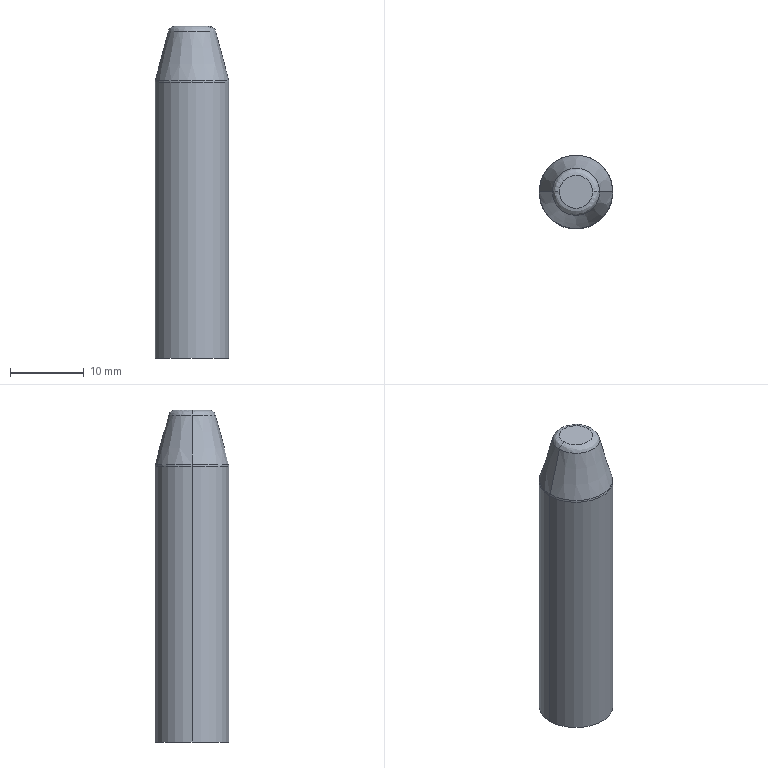Part | STEP file | Guard post | 1 solid | 13 faces | box 10 x 10 x 45 mm | volume 3034 mm3 | spline 4 | cylinder 4 | plane 3 | cone 2 | commonest cylinder face diameters 5 x2 10 x2
STEP:
#1=CARTESIAN_POINT('',(0.,0.,0.));
#2=DIRECTION('',(0.,0.,1.));
#3=DIRECTION('',(1.,0.,0.));
#4=AXIS2_PLACEMENT_3D('',#1,#2,#3);
#5=CARTESIAN_POINT('',(4.966,0.,37.663));
#6=VERTEX_POINT('',#5);
#7=CARTESIAN_POINT('',(-4.966,0.,37.663));
#8=VERTEX_POINT('',#7);
#9=CARTESIAN_POINT('',(0.,0.,37.663));
#10=DIRECTION('',(0.,0.,-1.));
#11=DIRECTION('',(1.,0.,0.));
#12=AXIS2_PLACEMENT_3D('',#9,#10,#11);
#13=CIRCLE('',#12,4.966);
#14=CARTESIAN_POINT('',(-4.966,0.,37.663));
#15=CARTESIAN_POINT('',(-4.966,-9.932,37.663));
#16=CARTESIAN_POINT('',(4.966,-9.932,37.663));
#17=CARTESIAN_POINT('',(4.966,0.,37.663));
#18=CARTESIAN_POINT('',(-4.989,0.,37.579));
#19=CARTESIAN_POINT('',(-4.989,-9.977,37.579));
#20=CARTESIAN_POINT('',(4.989,-9.977,37.579));
#21=CARTESIAN_POINT('',(4.989,0.,37.579));
#22=CARTESIAN_POINT('',(-5.,0.,37.492));
#23=CARTESIAN_POINT('',(-5.,-10.,37.492));
#24=CARTESIAN_POINT('',(5.,-10.,37.492));
#25=CARTESIAN_POINT('',(5.,0.,37.492));
#26=CARTESIAN_POINT('',(-5.,0.,37.404));
#27=CARTESIAN_POINT('',(-5.,-10.,37.404));
#28=CARTESIAN_POINT('',(5.,-10.,37.404));
#29=CARTESIAN_POINT('',(5.,0.,37.404));
#30=(BOUNDED_SURFACE()B_SPLINE_SURFACE(3,3,((#14,#15,#16,#17),(#18,#19,#20,#21),(#22,#23,#24,#25),(#26,#27,#28,#29)),.UNSPECIFIED.,.F.,.F.,.F.)B_SPLINE_SURFACE_WITH_KNOTS((4,4),(4,4),(0.,1.),(0.,1.),.PIECEWISE_BEZIER_KNOTS.)GEOMETRIC_REPRESENTATION_ITEM()RATIONAL_B_SPLINE_SURFACE(((1.,0.3333,0.3333,1.),(0.9943,0.3314,0.3314,0.9943),(0.9943,0.3314,0.3314,0.9943),(1.,0.3333,0.3333,1.)))REPRESENTATION_ITEM('')SURFACE());
#31=CARTESIAN_POINT('',(0.,1.));
#32=CARTESIAN_POINT('',(0.,0.9763));
#33=CARTESIAN_POINT('',(0.,0.9319));
#34=CARTESIAN_POINT('',(0.,0.8733));
#35=CARTESIAN_POINT('',(0.,0.8206));
#36=CARTESIAN_POINT('',(0.,0.7724));
#37=CARTESIAN_POINT('',(0.,0.7279));
#38=CARTESIAN_POINT('',(0.,0.6861));
#39=CARTESIAN_POINT('',(0.,0.6465));
#40=CARTESIAN_POINT('',(0.,0.6086));
#41=CARTESIAN_POINT('',(0.,0.5718));
#42=CARTESIAN_POINT('',(0.,0.5357));
#43=CARTESIAN_POINT('',(0.,0.5));
#44=CARTESIAN_POINT('',(0.,0.4643));
#45=CARTESIAN_POINT('',(0.,0.4282));
#46=CARTESIAN_POINT('',(0.,0.3914));
#47=CARTESIAN_POINT('',(0.,0.3535));
#48=CARTESIAN_POINT('',(0.,0.3139));
#49=CARTESIAN_POINT('',(0.,0.2721));
#50=CARTESIAN_POINT('',(0.,0.2276));
#51=CARTESIAN_POINT('',(0.,0.1794));
#52=CARTESIAN_POINT('',(0.,0.1267));
#53=CARTESIAN_POINT('',(0.,0.06805));
#54=CARTESIAN_POINT('',(0.,0.02375));
#55=CARTESIAN_POINT('',(0.,0.));
#56=B_SPLINE_CURVE_WITH_KNOTS('',3,(#31,#32,#33,#34,#35,#36,#37,#38,#39,#40,#41,#42,#43,#44,#45,#46,#47,#48,#49,#50,#51,#52,#53,#54,#55),.UNSPECIFIED.,.F.,.F.,(4,1,1,1,1,1,1,1,1,1,1,1,1,1,1,1,1,1,1,1,1,1,4),(0.,0.1428,0.2856,0.4284,0.5712,0.714,0.8568,0.9996,1.142,1.285,1.428,1.571,1.714,1.856,1.999,2.142,2.285,2.428,2.57,2.713,2.856,2.999,3.142),.QUASI_UNIFORM_KNOTS.);
#57=(GEOMETRIC_REPRESENTATION_CONTEXT(2)PARAMETRIC_REPRESENTATION_CONTEXT()REPRESENTATION_CONTEXT('',''));
#58=DEFINITIONAL_REPRESENTATION('',(#56),#57);
#59=PCURVE('',#30,#58);
#60=CARTESIAN_POINT('',(0.,0.,37.663));
#61=DIRECTION('',(0.,0.,-1.));
#62=DIRECTION('',(-1.,0.,0.));
#63=AXIS2_PLACEMENT_3D('',#60,#61,#62);
#64=CONICAL_SURFACE('',#63,4.966,0.2618);
#65=CARTESIAN_POINT('',(3.142,0.));
#66=DIRECTION('',(1.,0.));
#67=VECTOR('',#66,1.);
#68=LINE('',#65,#67);
#69=(GEOMETRIC_REPRESENTATION_CONTEXT(2)PARAMETRIC_REPRESENTATION_CONTEXT()REPRESENTATION_CONTEXT('',''));
#70=DEFINITIONAL_REPRESENTATION('',(#68),#69);
#71=PCURVE('',#64,#70);
#72=SURFACE_CURVE('',#13,(#59,#71),.PCURVE_S1.);
#73=EDGE_CURVE('',#6,#8,#72,.T.);
#74=ORIENTED_EDGE('',*,*,#73,.T.);
#75=CARTESIAN_POINT('',(-5.,0.,37.404));
#76=VERTEX_POINT('',#75);
#77=CARTESIAN_POINT('',(-4.,0.,37.404));
#78=DIRECTION('',(0.,-1.,0.));
#79=DIRECTION('',(-1.,0.,0.));
#80=AXIS2_PLACEMENT_3D('',#77,#78,#79);
#81=CIRCLE('',#80,1.);
#82=CARTESIAN_POINT('',(0.,0.));
#83=CARTESIAN_POINT('',(0.01519,0.));
#84=CARTESIAN_POINT('',(0.04557,0.));
#85=CARTESIAN_POINT('',(0.09111,0.));
#86=CARTESIAN_POINT('',(0.1366,0.));
#87=CARTESIAN_POINT('',(0.1821,0.));
#88=CARTESIAN_POINT('',(0.2275,0.));
#89=CARTESIAN_POINT('',(0.273,0.));
#90=CARTESIAN_POINT('',(0.3184,0.));
#91=CARTESIAN_POINT('',(0.3638,0.));
#92=CARTESIAN_POINT('',(0.4092,0.));
#93=CARTESIAN_POINT('',(0.4546,0.));
#94=CARTESIAN_POINT('',(0.5,0.));
#95=CARTESIAN_POINT('',(0.5454,0.));
#96=CARTESIAN_POINT('',(0.5908,0.));
#97=CARTESIAN_POINT('',(0.6362,0.));
#98=CARTESIAN_POINT('',(0.6816,0.));
#99=CARTESIAN_POINT('',(0.727,0.));
#100=CARTESIAN_POINT('',(0.7725,0.));
#101=CARTESIAN_POINT('',(0.8179,0.));
#102=CARTESIAN_POINT('',(0.8634,0.));
#103=CARTESIAN_POINT('',(0.9089,0.));
#104=CARTESIAN_POINT('',(0.9544,0.));
#105=CARTESIAN_POINT('',(0.9848,0.));
#106=CARTESIAN_POINT('',(1.,0.));
#107=B_SPLINE_CURVE_WITH_KNOTS('',3,(#82,#83,#84,#85,#86,#87,#88,#89,#90,#91,#92,#93,#94,#95,#96,#97,#98,#99,#100,#101,#102,#103,#104,#105,#106),.UNSPECIFIED.,.F.,.F.,(4,1,1,1,1,1,1,1,1,1,1,1,1,1,1,1,1,1,1,1,1,1,4),(6.021,6.033,6.045,6.057,6.069,6.081,6.093,6.105,6.117,6.128,6.14,6.152,6.164,6.176,6.188,6.2,6.212,6.224,6.236,6.247,6.259,6.271,6.283),.QUASI_UNIFORM_KNOTS.);
#108=(GEOMETRIC_REPRESENTATION_CONTEXT(2)PARAMETRIC_REPRESENTATION_CONTEXT()REPRESENTATION_CONTEXT('',''));
#109=DEFINITIONAL_REPRESENTATION('',(#107),#108);
#110=PCURVE('',#30,#109);
#111=CARTESIAN_POINT('',(4.966,0.,37.663));
#112=CARTESIAN_POINT('',(4.966,9.932,37.663));
#113=CARTESIAN_POINT('',(-4.966,9.932,37.663));
#114=CARTESIAN_POINT('',(-4.966,0.,37.663));
#115=CARTESIAN_POINT('',(4.989,0.,37.579));
#116=CARTESIAN_POINT('',(4.989,9.977,37.579));
#117=CARTESIAN_POINT('',(-4.989,9.977,37.579));
#118=CARTESIAN_POINT('',(-4.989,0.,37.579));
#119=CARTESIAN_POINT('',(5.,0.,37.492));
#120=CARTESIAN_POINT('',(5.,10.,37.492));
#121=CARTESIAN_POINT('',(-5.,10.,37.492));
#122=CARTESIAN_POINT('',(-5.,0.,37.492));
#123=CARTESIAN_POINT('',(5.,0.,37.404));
#124=CARTESIAN_POINT('',(5.,10.,37.404));
#125=CARTESIAN_POINT('',(-5.,10.,37.404));
#126=CARTESIAN_POINT('',(-5.,0.,37.404));
#127=(BOUNDED_SURFACE()B_SPLINE_SURFACE(3,3,((#111,#112,#113,#114),(#115,#116,#117,#118),(#119,#120,#121,#122),(#123,#124,#125,#126)),.UNSPECIFIED.,.F.,.F.,.F.)B_SPLINE_SURFACE_WITH_KNOTS((4,4),(4,4),(0.,1.),(0.,1.),.PIECEWISE_BEZIER_KNOTS.)GEOMETRIC_REPRESENTATION_ITEM()RATIONAL_B_SPLINE_SURFACE(((1.,0.3333,0.3333,1.),(0.9943,0.3314,0.3314,0.9943),(0.9943,0.3314,0.3314,0.9943),(1.,0.3333,0.3333,1.)))REPRESENTATION_ITEM('')SURFACE());
#128=CARTESIAN_POINT('',(0.,1.));
#129=CARTESIAN_POINT('',(0.01519,1.));
#130=CARTESIAN_POINT('',(0.04557,1.));
#131=CARTESIAN_POINT('',(0.09111,1.));
#132=CARTESIAN_POINT('',(0.1366,1.));
#133=CARTESIAN_POINT('',(0.1821,1.));
#134=CARTESIAN_POINT('',(0.2275,1.));
#135=CARTESIAN_POINT('',(0.273,1.));
#136=CARTESIAN_POINT('',(0.3184,1.));
#137=CARTESIAN_POINT('',(0.3638,1.));
#138=CARTESIAN_POINT('',(0.4092,1.));
#139=CARTESIAN_POINT('',(0.4546,1.));
#140=CARTESIAN_POINT('',(0.5,1.));
#141=CARTESIAN_POINT('',(0.5454,1.));
#142=CARTESIAN_POINT('',(0.5908,1.));
#143=CARTESIAN_POINT('',(0.6362,1.));
#144=CARTESIAN_POINT('',(0.6816,1.));
#145=CARTESIAN_POINT('',(0.727,1.));
#146=CARTESIAN_POINT('',(0.7725,1.));
#147=CARTESIAN_POINT('',(0.8179,1.));
#148=CARTESIAN_POINT('',(0.8634,1.));
#149=CARTESIAN_POINT('',(0.9089,1.));
#150=CARTESIAN_POINT('',(0.9544,1.));
#151=CARTESIAN_POINT('',(0.9848,1.));
#152=CARTESIAN_POINT('',(1.,1.));
#153=B_SPLINE_CURVE_WITH_KNOTS('',3,(#128,#129,#130,#131,#132,#133,#134,#135,#136,#137,#138,#139,#140,#141,#142,#143,#144,#145,#146,#147,#148,#149,#150,#151,#152),.UNSPECIFIED.,.F.,.F.,(4,1,1,1,1,1,1,1,1,1,1,1,1,1,1,1,1,1,1,1,1,1,4),(6.021,6.033,6.045,6.057,6.069,6.081,6.093,6.105,6.117,6.128,6.14,6.152,6.164,6.176,6.188,6.2,6.212,6.224,6.236,6.247,6.259,6.271,6.283),.QUASI_UNIFORM_KNOTS.);
#154=(GEOMETRIC_REPRESENTATION_CONTEXT(2)PARAMETRIC_REPRESENTATION_CONTEXT()REPRESENTATION_CONTEXT('',''));
#155=DEFINITIONAL_REPRESENTATION('',(#153),#154);
#156=PCURVE('',#127,#155);
#157=SURFACE_CURVE('',#81,(#110,#156),.PCURVE_S1.);
#158=EDGE_CURVE('',#8,#76,#157,.T.);
#159=ORIENTED_EDGE('',*,*,#158,.T.);
#160=CARTESIAN_POINT('',(5.,0.,37.404));
#161=VERTEX_POINT('',#160);
#162=CARTESIAN_POINT('',(0.,0.,37.404));
#163=DIRECTION('',(0.,0.,-1.));
#164=DIRECTION('',(-1.,0.,0.));
#165=AXIS2_PLACEMENT_3D('',#162,#163,#164);
#166=CIRCLE('',#165,5.);
#167=CARTESIAN_POINT('',(1.,1.));
#168=CARTESIAN_POINT('',(1.,0.9763));
#169=CARTESIAN_POINT('',(1.,0.9319));
#170=CARTESIAN_POINT('',(1.,0.8733));
#171=CARTESIAN_POINT('',(1.,0.8206));
#172=CARTESIAN_POINT('',(1.,0.7724));
#173=CARTESIAN_POINT('',(1.,0.7279));
#174=CARTESIAN_POINT('',(1.,0.6861));
#175=CARTESIAN_POINT('',(1.,0.6465));
#176=CARTESIAN_POINT('',(1.,0.6086));
#177=CARTESIAN_POINT('',(1.,0.5718));
#178=CARTESIAN_POINT('',(1.,0.5357));
#179=CARTESIAN_POINT('',(1.,0.5));
#180=CARTESIAN_POINT('',(1.,0.4643));
#181=CARTESIAN_POINT('',(1.,0.4282));
#182=CARTESIAN_POINT('',(1.,0.3914));
#183=CARTESIAN_POINT('',(1.,0.3535));
#184=CARTESIAN_POINT('',(1.,0.3139));
#185=CARTESIAN_POINT('',(1.,0.2721));
#186=CARTESIAN_POINT('',(1.,0.2276));
#187=CARTESIAN_POINT('',(1.,0.1794));
#188=CARTESIAN_POINT('',(1.,0.1267));
#189=CARTESIAN_POINT('',(1.,0.06805));
#190=CARTESIAN_POINT('',(1.,0.02375));
#191=CARTESIAN_POINT('',(1.,0.));
#192=B_SPLINE_CURVE_WITH_KNOTS('',3,(#167,#168,#169,#170,#171,#172,#173,#174,#175,#176,#177,#178,#179,#180,#181,#182,#183,#184,#185,#186,#187,#188,#189,#190,#191),.UNSPECIFIED.,.F.,.F.,(4,1,1,1,1,1,1,1,1,1,1,1,1,1,1,1,1,1,1,1,1,1,4),(3.142,3.284,3.427,3.57,3.713,3.856,3.998,4.141,4.284,4.427,4.57,4.712,4.855,4.998,5.141,5.284,5.426,5.569,5.712,5.855,5.998,6.14,6.283),.QUASI_UNIFORM_KNOTS.);
#193=(GEOMETRIC_REPRESENTATION_CONTEXT(2)PARAMETRIC_REPRESENTATION_CONTEXT()REPRESENTATION_CONTEXT('',''));
#194=DEFINITIONAL_REPRESENTATION('',(#192),#193);
#195=PCURVE('',#30,#194);
#196=CARTESIAN_POINT('',(0.,0.,45.));
#197=DIRECTION('',(0.,0.,-1.));
#198=DIRECTION('',(-1.,0.,0.));
#199=AXIS2_PLACEMENT_3D('',#196,#197,#198);
#200=CYLINDRICAL_SURFACE('',#199,5.);
#201=CARTESIAN_POINT('',(0.,7.596));
#202=DIRECTION('',(1.,0.));
#203=VECTOR('',#202,1.);
#204=LINE('',#201,#203);
#205=(GEOMETRIC_REPRESENTATION_CONTEXT(2)PARAMETRIC_REPRESENTATION_CONTEXT()REPRESENTATION_CONTEXT('',''));
#206=DEFINITIONAL_REPRESENTATION('',(#204),#205);
#207=PCURVE('',#200,#206);
#208=SURFACE_CURVE('',#166,(#195,#207),.PCURVE_S1.);
#209=EDGE_CURVE('',#161,#76,#208,.T.);
#210=ORIENTED_EDGE('',*,*,#209,.F.);
#211=CARTESIAN_POINT('',(4.,0.,37.404));
#212=DIRECTION('',(0.,1.,0.));
#213=DIRECTION('',(1.,0.,0.));
#214=AXIS2_PLACEMENT_3D('',#211,#212,#213);
#215=CIRCLE('',#214,1.);
#216=CARTESIAN_POINT('',(0.,1.));
#217=CARTESIAN_POINT('',(0.01519,1.));
#218=CARTESIAN_POINT('',(0.04557,1.));
#219=CARTESIAN_POINT('',(0.09111,1.));
#220=CARTESIAN_POINT('',(0.1366,1.));
#221=CARTESIAN_POINT('',(0.1821,1.));
#222=CARTESIAN_POINT('',(0.2275,1.));
#223=CARTESIAN_POINT('',(0.273,1.));
#224=CARTESIAN_POINT('',(0.3184,1.));
#225=CARTESIAN_POINT('',(0.3638,1.));
#226=CARTESIAN_POINT('',(0.4092,1.));
#227=CARTESIAN_POINT('',(0.4546,1.));
#228=CARTESIAN_POINT('',(0.5,1.));
#229=CARTESIAN_POINT('',(0.5454,1.));
#230=CARTESIAN_POINT('',(0.5908,1.));
#231=CARTESIAN_POINT('',(0.6362,1.));
#232=CARTESIAN_POINT('',(0.6816,1.));
#233=CARTESIAN_POINT('',(0.727,1.));
#234=CARTESIAN_POINT('',(0.7725,1.));
#235=CARTESIAN_POINT('',(0.8179,1.));
#236=CARTESIAN_POINT('',(0.8634,1.));
#237=CARTESIAN_POINT('',(0.9089,1.));
#238=CARTESIAN_POINT('',(0.9544,1.));
#239=CARTESIAN_POINT('',(0.9848,1.));
#240=CARTESIAN_POINT('',(1.,1.));
#241=B_SPLINE_CURVE_WITH_KNOTS('',3,(#216,#217,#218,#219,#220,#221,#222,#223,#224,#225,#226,#227,#228,#229,#230,#231,#232,#233,#234,#235,#236,#237,#238,#239,#240),.UNSPECIFIED.,.F.,.F.,(4,1,1,1,1,1,1,1,1,1,1,1,1,1,1,1,1,1,1,1,1,1,4),(6.021,6.033,6.045,6.057,6.069,6.081,6.093,6.105,6.117,6.128,6.14,6.152,6.164,6.176,6.188,6.2,6.212,6.224,6.236,6.247,6.259,6.271,6.283),.QUASI_UNIFORM_KNOTS.);
#242=(GEOMETRIC_REPRESENTATION_CONTEXT(2)PARAMETRIC_REPRESENTATION_CONTEXT()REPRESENTATION_CONTEXT('',''));
#243=DEFINITIONAL_REPRESENTATION('',(#241),#242);
#244=PCURVE('',#30,#243);
#245=CARTESIAN_POINT('',(0.,0.));
#246=CARTESIAN_POINT('',(0.01519,0.));
#247=CARTESIAN_POINT('',(0.04557,0.));
#248=CARTESIAN_POINT('',(0.09111,0.));
#249=CARTESIAN_POINT('',(0.1366,0.));
#250=CARTESIAN_POINT('',(0.1821,0.));
#251=CARTESIAN_POINT('',(0.2275,0.));
#252=CARTESIAN_POINT('',(0.273,0.));
#253=CARTESIAN_POINT('',(0.3184,0.));
#254=CARTESIAN_POINT('',(0.3638,0.));
#255=CARTESIAN_POINT('',(0.4092,0.));
#256=CARTESIAN_POINT('',(0.4546,0.));
#257=CARTESIAN_POINT('',(0.5,0.));
#258=CARTESIAN_POINT('',(0.5454,0.));
#259=CARTESIAN_POINT('',(0.5908,0.));
#260=CARTESIAN_POINT('',(0.6362,0.));
#261=CARTESIAN_POINT('',(0.6816,0.));
#262=CARTESIAN_POINT('',(0.727,0.));
#263=CARTESIAN_POINT('',(0.7725,0.));
#264=CARTESIAN_POINT('',(0.8179,0.));
#265=CARTESIAN_POINT('',(0.8634,0.));
#266=CARTESIAN_POINT('',(0.9089,0.));
#267=CARTESIAN_POINT('',(0.9544,0.));
#268=CARTESIAN_POINT('',(0.9848,0.));
#269=CARTESIAN_POINT('',(1.,0.));
#270=B_SPLINE_CURVE_WITH_KNOTS('',3,(#245,#246,#247,#248,#249,#250,#251,#252,#253,#254,#255,#256,#257,#258,#259,#260,#261,#262,#263,#264,#265,#266,#267,#268,#269),.UNSPECIFIED.,.F.,.F.,(4,1,1,1,1,1,1,1,1,1,1,1,1,1,1,1,1,1,1,1,1,1,4),(6.021,6.033,6.045,6.057,6.069,6.081,6.093,6.105,6.117,6.128,6.14,6.152,6.164,6.176,6.188,6.2,6.212,6.224,6.236,6.247,6.259,6.271,6.283),.QUASI_UNIFORM_KNOTS.);
#271=(GEOMETRIC_REPRESENTATION_CONTEXT(2)PARAMETRIC_REPRESENTATION_CONTEXT()REPRESENTATION_CONTEXT('',''));
#272=DEFINITIONAL_REPRESENTATION('',(#270),#271);
#273=PCURVE('',#127,#272);
#274=SURFACE_CURVE('',#215,(#244,#273),.PCURVE_S1.);
#275=EDGE_CURVE('',#6,#161,#274,.T.);
#276=ORIENTED_EDGE('',*,*,#275,.F.);
#277=EDGE_LOOP('',(#74,#159,#210,#276));
#278=FACE_BOUND('',#277,.T.);
#279=ADVANCED_FACE('',(#278),#30,.T.);
#280=CARTESIAN_POINT('',(2.233,0.,45.));
#281=VERTEX_POINT('',#280);
#282=CARTESIAN_POINT('',(-2.233,0.,45.));
#283=VERTEX_POINT('',#282);
#284=CARTESIAN_POINT('',(2.233,0.,45.));
#285=CARTESIAN_POINT('',(2.233,-4.465,45.));
#286=CARTESIAN_POINT('',(-2.233,-4.465,45.));
#287=CARTESIAN_POINT('',(-2.233,0.,45.));
#288=(BOUNDED_CURVE()B_SPLINE_CURVE(3,(#284,#285,#286,#287),.UNSPECIFIED.,.F.,.F.)B_SPLINE_CURVE_WITH_KNOTS((4,4),(0.,1.),.PIECEWISE_BEZIER_KNOTS.)CURVE()GEOMETRIC_REPRESENTATION_ITEM()RATIONAL_B_SPLINE_CURVE((1.,0.3333,0.3333,1.))REPRESENTATION_ITEM(''));
#289=CARTESIAN_POINT('',(-2.233,0.,45.));
#290=CARTESIAN_POINT('',(-2.233,-4.465,45.));
#291=CARTESIAN_POINT('',(2.233,-4.465,45.));
#292=CARTESIAN_POINT('',(2.233,0.,45.));
#293=CARTESIAN_POINT('',(-2.703,0.,45.));
#294=CARTESIAN_POINT('',(-2.703,-5.407,45.));
#295=CARTESIAN_POINT('',(2.703,-5.407,45.));
#296=CARTESIAN_POINT('',(2.703,0.,45.));
#297=CARTESIAN_POINT('',(-3.077,0.,44.713));
#298=CARTESIAN_POINT('',(-3.077,-6.154,44.713));
#299=CARTESIAN_POINT('',(3.077,-6.154,44.713));
#300=CARTESIAN_POINT('',(3.077,0.,44.713));
#301=CARTESIAN_POINT('',(-3.199,0.,44.259));
#302=CARTESIAN_POINT('',(-3.199,-6.397,44.259));
#303=CARTESIAN_POINT('',(3.199,-6.397,44.259));
#304=CARTESIAN_POINT('',(3.199,0.,44.259));
#305=(BOUNDED_SURFACE()B_SPLINE_SURFACE(3,3,((#289,#290,#291,#292),(#293,#294,#295,#296),(#297,#298,#299,#300),(#301,#302,#303,#304)),.UNSPECIFIED.,.F.,.F.,.F.)B_SPLINE_SURFACE_WITH_KNOTS((4,4),(4,4),(0.,1.),(0.,1.),.PIECEWISE_BEZIER_KNOTS.)GEOMETRIC_REPRESENTATION_ITEM()RATIONAL_B_SPLINE_SURFACE(((1.,0.3333,0.3333,1.),(0.8622,0.2874,0.2874,0.8622),(0.8622,0.2874,0.2874,0.8622),(1.,0.3333,0.3333,1.)))REPRESENTATION_ITEM('')SURFACE());
#306=CARTESIAN_POINT('',(0.,1.));
#307=DIRECTION('',(0.,-1.));
#308=VECTOR('',#307,1.);
#309=LINE('',#306,#308);
#310=(GEOMETRIC_REPRESENTATION_CONTEXT(2)PARAMETRIC_REPRESENTATION_CONTEXT()REPRESENTATION_CONTEXT('',''));
#311=DEFINITIONAL_REPRESENTATION('',(#309),#310);
#312=PCURVE('',#305,#311);
#313=CARTESIAN_POINT('',(0.,0.,45.));
#314=DIRECTION('',(0.,0.,1.));
#315=DIRECTION('',(1.,0.,0.));
#316=AXIS2_PLACEMENT_3D('',#313,#314,#315);
#317=PLANE('',#316);
#318=CARTESIAN_POINT('',(2.233,0.));
#319=CARTESIAN_POINT('',(2.233,-4.465));
#320=CARTESIAN_POINT('',(-2.233,-4.465));
#321=CARTESIAN_POINT('',(-2.233,0.));
#322=(BOUNDED_CURVE()B_SPLINE_CURVE(3,(#318,#319,#320,#321),.UNSPECIFIED.,.F.,.F.)B_SPLINE_CURVE_WITH_KNOTS((4,4),(0.,1.),.PIECEWISE_BEZIER_KNOTS.)CURVE()GEOMETRIC_REPRESENTATION_ITEM()RATIONAL_B_SPLINE_CURVE((1.,0.3333,0.3333,1.))REPRESENTATION_ITEM(''));
#323=(GEOMETRIC_REPRESENTATION_CONTEXT(2)PARAMETRIC_REPRESENTATION_CONTEXT()REPRESENTATION_CONTEXT('',''));
#324=DEFINITIONAL_REPRESENTATION('',(#322),#323);
#325=PCURVE('',#317,#324);
#326=SURFACE_CURVE('',#288,(#312,#325),.PCURVE_S1.);
#327=EDGE_CURVE('',#281,#283,#326,.T.);
#328=ORIENTED_EDGE('',*,*,#327,.T.);
#329=CARTESIAN_POINT('',(-3.199,0.,44.259));
#330=VERTEX_POINT('',#329);
#331=CARTESIAN_POINT('',(-2.233,0.,44.));
#332=DIRECTION('',(0.,-1.,0.));
#333=DIRECTION('',(-1.,0.,0.));
#334=AXIS2_PLACEMENT_3D('',#331,#332,#333);
#335=CIRCLE('',#334,1.);
#336=CARTESIAN_POINT('',(0.,0.));
#337=CARTESIAN_POINT('',(0.01629,0.));
#338=CARTESIAN_POINT('',(0.04854,0.));
#339=CARTESIAN_POINT('',(0.09604,0.));
#340=CARTESIAN_POINT('',(0.1428,0.));
#341=CARTESIAN_POINT('',(0.1888,0.));
#342=CARTESIAN_POINT('',(0.2343,0.));
#343=CARTESIAN_POINT('',(0.2793,0.));
#344=CARTESIAN_POINT('',(0.3239,0.));
#345=CARTESIAN_POINT('',(0.3682,0.));
#346=CARTESIAN_POINT('',(0.4123,0.));
#347=CARTESIAN_POINT('',(0.4562,0.));
#348=CARTESIAN_POINT('',(0.5,0.));
#349=CARTESIAN_POINT('',(0.5438,0.));
#350=CARTESIAN_POINT('',(0.5877,0.));
#351=CARTESIAN_POINT('',(0.6318,0.));
#352=CARTESIAN_POINT('',(0.6761,0.));
#353=CARTESIAN_POINT('',(0.7207,0.));
#354=CARTESIAN_POINT('',(0.7657,0.));
#355=CARTESIAN_POINT('',(0.8112,0.));
#356=CARTESIAN_POINT('',(0.8572,0.));
#357=CARTESIAN_POINT('',(0.904,0.));
#358=CARTESIAN_POINT('',(0.9515,0.));
#359=CARTESIAN_POINT('',(0.9837,0.));
#360=CARTESIAN_POINT('',(1.,0.));
#361=B_SPLINE_CURVE_WITH_KNOTS('',3,(#336,#337,#338,#339,#340,#341,#342,#343,#344,#345,#346,#347,#348,#349,#350,#351,#352,#353,#354,#355,#356,#357,#358,#359,#360),.UNSPECIFIED.,.F.,.F.,(4,1,1,1,1,1,1,1,1,1,1,1,1,1,1,1,1,1,1,1,1,1,4),(4.712,4.772,4.831,4.891,4.95,5.01,5.069,5.129,5.188,5.248,5.307,5.367,5.426,5.486,5.545,5.605,5.664,5.724,5.783,5.843,5.902,5.962,6.021),.QUASI_UNIFORM_KNOTS.);
#362=(GEOMETRIC_REPRESENTATION_CONTEXT(2)PARAMETRIC_REPRESENTATION_CONTEXT()REPRESENTATION_CONTEXT('',''));
#363=DEFINITIONAL_REPRESENTATION('',(#361),#362);
#364=PCURVE('',#305,#363);
#365=CARTESIAN_POINT('',(2.233,0.,45.));
#366=CARTESIAN_POINT('',(2.233,4.465,45.));
#367=CARTESIAN_POINT('',(-2.233,4.465,45.));
#368=CARTESIAN_POINT('',(-2.233,0.,45.));
#369=CARTESIAN_POINT('',(2.703,0.,45.));
#370=CARTESIAN_POINT('',(2.703,5.407,45.));
#371=CARTESIAN_POINT('',(-2.703,5.407,45.));
#372=CARTESIAN_POINT('',(-2.703,0.,45.));
#373=CARTESIAN_POINT('',(3.077,0.,44.713));
#374=CARTESIAN_POINT('',(3.077,6.154,44.713));
#375=CARTESIAN_POINT('',(-3.077,6.154,44.713));
#376=CARTESIAN_POINT('',(-3.077,0.,44.713));
#377=CARTESIAN_POINT('',(3.199,0.,44.259));
#378=CARTESIAN_POINT('',(3.199,6.397,44.259));
#379=CARTESIAN_POINT('',(-3.199,6.397,44.259));
#380=CARTESIAN_POINT('',(-3.199,0.,44.259));
#381=(BOUNDED_SURFACE()B_SPLINE_SURFACE(3,3,((#365,#366,#367,#368),(#369,#370,#371,#372),(#373,#374,#375,#376),(#377,#378,#379,#380)),.UNSPECIFIED.,.F.,.F.,.F.)B_SPLINE_SURFACE_WITH_KNOTS((4,4),(4,4),(0.,1.),(0.,1.),.PIECEWISE_BEZIER_KNOTS.)GEOMETRIC_REPRESENTATION_ITEM()RATIONAL_B_SPLINE_SURFACE(((1.,0.3333,0.3333,1.),(0.8622,0.2874,0.2874,0.8622),(0.8622,0.2874,0.2874,0.8622),(1.,0.3333,0.3333,1.)))REPRESENTATION_ITEM('')SURFACE());
#382=CARTESIAN_POINT('',(0.,1.));
#383=CARTESIAN_POINT('',(0.01629,1.));
#384=CARTESIAN_POINT('',(0.04854,1.));
#385=CARTESIAN_POINT('',(0.09604,1.));
#386=CARTESIAN_POINT('',(0.1428,1.));
#387=CARTESIAN_POINT('',(0.1888,1.));
#388=CARTESIAN_POINT('',(0.2343,1.));
#389=CARTESIAN_POINT('',(0.2793,1.));
#390=CARTESIAN_POINT('',(0.3239,1.));
#391=CARTESIAN_POINT('',(0.3682,1.));
#392=CARTESIAN_POINT('',(0.4123,1.));
#393=CARTESIAN_POINT('',(0.4562,1.));
#394=CARTESIAN_POINT('',(0.5,1.));
#395=CARTESIAN_POINT('',(0.5438,1.));
#396=CARTESIAN_POINT('',(0.5877,1.));
#397=CARTESIAN_POINT('',(0.6318,1.));
#398=CARTESIAN_POINT('',(0.6761,1.));
#399=CARTESIAN_POINT('',(0.7207,1.));
#400=CARTESIAN_POINT('',(0.7657,1.));
#401=CARTESIAN_POINT('',(0.8112,1.));
#402=CARTESIAN_POINT('',(0.8572,1.));
#403=CARTESIAN_POINT('',(0.904,1.));
#404=CARTESIAN_POINT('',(0.9515,1.));
#405=CARTESIAN_POINT('',(0.9837,1.));
#406=CARTESIAN_POINT('',(1.,1.));
#407=B_SPLINE_CURVE_WITH_KNOTS('',3,(#382,#383,#384,#385,#386,#387,#388,#389,#390,#391,#392,#393,#394,#395,#396,#397,#398,#399,#400,#401,#402,#403,#404,#405,#406),.UNSPECIFIED.,.F.,.F.,(4,1,1,1,1,1,1,1,1,1,1,1,1,1,1,1,1,1,1,1,1,1,4),(4.712,4.772,4.831,4.891,4.95,5.01,5.069,5.129,5.188,5.248,5.307,5.367,5.426,5.486,5.545,5.605,5.664,5.724,5.783,5.843,5.902,5.962,6.021),.QUASI_UNIFORM_KNOTS.);
#408=(GEOMETRIC_REPRESENTATION_CONTEXT(2)PARAMETRIC_REPRESENTATION_CONTEXT()REPRESENTATION_CONTEXT('',''));
#409=DEFINITIONAL_REPRESENTATION('',(#407),#408);
#410=PCURVE('',#381,#409);
#411=SURFACE_CURVE('',#335,(#364,#410),.PCURVE_S1.);
#412=EDGE_CURVE('',#283,#330,#411,.T.);
#413=ORIENTED_EDGE('',*,*,#412,.T.);
#414=CARTESIAN_POINT('',(3.199,0.,44.259));
#415=VERTEX_POINT('',#414);
#416=CARTESIAN_POINT('',(0.,0.,44.259));
#417=DIRECTION('',(0.,0.,-1.));
#418=DIRECTION('',(-1.,0.,0.));
#419=AXIS2_PLACEMENT_3D('',#416,#417,#418);
#420=CIRCLE('',#419,3.199);
#421=CARTESIAN_POINT('',(1.,1.));
#422=CARTESIAN_POINT('',(1.,0.9763));
#423=CARTESIAN_POINT('',(1.,0.9319));
#424=CARTESIAN_POINT('',(1.,0.8733));
#425=CARTESIAN_POINT('',(1.,0.8206));
#426=CARTESIAN_POINT('',(1.,0.7724));
#427=CARTESIAN_POINT('',(1.,0.7279));
#428=CARTESIAN_POINT('',(1.,0.6861));
#429=CARTESIAN_POINT('',(1.,0.6465));
#430=CARTESIAN_POINT('',(1.,0.6086));
#431=CARTESIAN_POINT('',(1.,0.5718));
#432=CARTESIAN_POINT('',(1.,0.5357));
#433=CARTESIAN_POINT('',(1.,0.5));
#434=CARTESIAN_POINT('',(1.,0.4643));
#435=CARTESIAN_POINT('',(1.,0.4282));
#436=CARTESIAN_POINT('',(1.,0.3914));
#437=CARTESIAN_POINT('',(1.,0.3535));
#438=CARTESIAN_POINT('',(1.,0.3139));
#439=CARTESIAN_POINT('',(1.,0.2721));
#440=CARTESIAN_POINT('',(1.,0.2276));
#441=CARTESIAN_POINT('',(1.,0.1794));
#442=CARTESIAN_POINT('',(1.,0.1267));
#443=CARTESIAN_POINT('',(1.,0.06805));
#444=CARTESIAN_POINT('',(1.,0.02375));
#445=CARTESIAN_POINT('',(1.,0.));
#446=B_SPLINE_CURVE_WITH_KNOTS('',3,(#421,#422,#423,#424,#425,#426,#427,#428,#429,#430,#431,#432,#433,#434,#435,#436,#437,#438,#439,#440,#441,#442,#443,#444,#445),.UNSPECIFIED.,.F.,.F.,(4,1,1,1,1,1,1,1,1,1,1,1,1,1,1,1,1,1,1,1,1,1,4),(3.142,3.284,3.427,3.57,3.713,3.856,3.998,4.141,4.284,4.427,4.57,4.712,4.855,4.998,5.141,5.284,5.426,5.569,5.712,5.855,5.998,6.14,6.283),.QUASI_UNIFORM_KNOTS.);
#447=(GEOMETRIC_REPRESENTATION_CONTEXT(2)PARAMETRIC_REPRESENTATION_CONTEXT()REPRESENTATION_CONTEXT('',''));
#448=DEFINITIONAL_REPRESENTATION('',(#446),#447);
#449=PCURVE('',#305,#448);
#450=CARTESIAN_POINT('',(0.,-6.596));
#451=DIRECTION('',(1.,0.));
#452=VECTOR('',#451,1.);
#453=LINE('',#450,#452);
#454=(GEOMETRIC_REPRESENTATION_CONTEXT(2)PARAMETRIC_REPRESENTATION_CONTEXT()REPRESENTATION_CONTEXT('',''));
#455=DEFINITIONAL_REPRESENTATION('',(#453),#454);
#456=PCURVE('',#64,#455);
#457=SURFACE_CURVE('',#420,(#449,#456),.PCURVE_S1.);
#458=EDGE_CURVE('',#415,#330,#457,.T.);
#459=ORIENTED_EDGE('',*,*,#458,.F.);
#460=CARTESIAN_POINT('',(2.233,0.,44.));
#461=DIRECTION('',(0.,1.,0.));
#462=DIRECTION('',(1.,0.,0.));
#463=AXIS2_PLACEMENT_3D('',#460,#461,#462);
#464=CIRCLE('',#463,1.);
#465=CARTESIAN_POINT('',(0.,1.));
#466=CARTESIAN_POINT('',(0.01629,1.));
#467=CARTESIAN_POINT('',(0.04854,1.));
#468=CARTESIAN_POINT('',(0.09604,1.));
#469=CARTESIAN_POINT('',(0.1428,1.));
#470=CARTESIAN_POINT('',(0.1888,1.));
#471=CARTESIAN_POINT('',(0.2343,1.));
#472=CARTESIAN_POINT('',(0.2793,1.));
#473=CARTESIAN_POINT('',(0.3239,1.));
#474=CARTESIAN_POINT('',(0.3682,1.));
#475=CARTESIAN_POINT('',(0.4123,1.));
#476=CARTESIAN_POINT('',(0.4562,1.));
#477=CARTESIAN_POINT('',(0.5,1.));
#478=CARTESIAN_POINT('',(0.5438,1.));
#479=CARTESIAN_POINT('',(0.5877,1.));
#480=CARTESIAN_POINT('',(0.6318,1.));
#481=CARTESIAN_POINT('',(0.6761,1.));
#482=CARTESIAN_POINT('',(0.7207,1.));
#483=CARTESIAN_POINT('',(0.7657,1.));
#484=CARTESIAN_POINT('',(0.8112,1.));
#485=CARTESIAN_POINT('',(0.8572,1.));
#486=CARTESIAN_POINT('',(0.904,1.));
#487=CARTESIAN_POINT('',(0.9515,1.));
#488=CARTESIAN_POINT('',(0.9837,1.));
#489=CARTESIAN_POINT('',(1.,1.));
#490=B_SPLINE_CURVE_WITH_KNOTS('',3,(#465,#466,#467,#468,#469,#470,#471,#472,#473,#474,#475,#476,#477,#478,#479,#480,#481,#482,#483,#484,#485,#486,#487,#488,#489),.UNSPECIFIED.,.F.,.F.,(4,1,1,1,1,1,1,1,1,1,1,1,1,1,1,1,1,1,1,1,1,1,4),(4.712,4.772,4.831,4.891,4.95,5.01,5.069,5.129,5.188,5.248,5.307,5.367,5.426,5.486,5.545,5.605,5.664,5.724,5.783,5.843,5.902,5.962,6.021),.QUASI_UNIFORM_KNOTS.);
#491=(GEOMETRIC_REPRESENTATION_CONTEXT(2)PARAMETRIC_REPRESENTATION_CONTEXT()REPRESENTATION_CONTEXT('',''));
#492=DEFINITIONAL_REPRESENTATION('',(#490),#491);
#493=PCURVE('',#305,#492);
#494=CARTESIAN_POINT('',(0.,0.));
#495=CARTESIAN_POINT('',(0.01629,0.));
#496=CARTESIAN_POINT('',(0.04854,0.));
#497=CARTESIAN_POINT('',(0.09604,0.));
#498=CARTESIAN_POINT('',(0.1428,0.));
#499=CARTESIAN_POINT('',(0.1888,0.));
#500=CARTESIAN_POINT('',(0.2343,0.));
#501=CARTESIAN_POINT('',(0.2793,0.));
#502=CARTESIAN_POINT('',(0.3239,0.));
#503=CARTESIAN_POINT('',(0.3682,0.));
#504=CARTESIAN_POINT('',(0.4123,0.));
#505=CARTESIAN_POINT('',(0.4562,0.));
#506=CARTESIAN_POINT('',(0.5,0.));
#507=CARTESIAN_POINT('',(0.5438,0.));
#508=CARTESIAN_POINT('',(0.5877,0.));
#509=CARTESIAN_POINT('',(0.6318,0.));
#510=CARTESIAN_POINT('',(0.6761,0.));
#511=CARTESIAN_POINT('',(0.7207,0.));
#512=CARTESIAN_POINT('',(0.7657,0.));
#513=CARTESIAN_POINT('',(0.8112,0.));
#514=CARTESIAN_POINT('',(0.8572,0.));
#515=CARTESIAN_POINT('',(0.904,0.));
#516=CARTESIAN_POINT('',(0.9515,0.));
#517=CARTESIAN_POINT('',(0.9837,0.));
#518=CARTESIAN_POINT('',(1.,0.));
#519=B_SPLINE_CURVE_WITH_KNOTS('',3,(#494,#495,#496,#497,#498,#499,#500,#501,#502,#503,#504,#505,#506,#507,#508,#509,#510,#511,#512,#513,#514,#515,#516,#517,#518),.UNSPECIFIED.,.F.,.F.,(4,1,1,1,1,1,1,1,1,1,1,1,1,1,1,1,1,1,1,1,1,1,4),(4.712,4.772,4.831,4.891,4.95,5.01,5.069,5.129,5.188,5.248,5.307,5.367,5.426,5.486,5.545,5.605,5.664,5.724,5.783,5.843,5.902,5.962,6.021),.QUASI_UNIFORM_KNOTS.);
#520=(GEOMETRIC_REPRESENTATION_CONTEXT(2)PARAMETRIC_REPRESENTATION_CONTEXT()REPRESENTATION_CONTEXT('',''));
#521=DEFINITIONAL_REPRESENTATION('',(#519),#520);
#522=PCURVE('',#381,#521);
#523=SURFACE_CURVE('',#464,(#493,#522),.PCURVE_S1.);
#524=EDGE_CURVE('',#281,#415,#523,.T.);
#525=ORIENTED_EDGE('',*,*,#524,.F.);
#526=EDGE_LOOP('',(#328,#413,#459,#525));
#527=FACE_BOUND('',#526,.T.);
#528=ADVANCED_FACE('',(#527),#305,.T.);
#529=CARTESIAN_POINT('',(0.,0.,37.404));
#530=DIRECTION('',(0.,0.,-1.));
#531=DIRECTION('',(-1.,0.,0.));
#532=AXIS2_PLACEMENT_3D('',#529,#530,#531);
#533=CIRCLE('',#532,5.);
#534=CARTESIAN_POINT('',(0.,0.,45.));
#535=DIRECTION('',(0.,0.,-1.));
#536=DIRECTION('',(-1.,0.,0.));
#537=AXIS2_PLACEMENT_3D('',#534,#535,#536);
#538=CYLINDRICAL_SURFACE('',#537,5.);
#539=CARTESIAN_POINT('',(0.,7.596));
#540=DIRECTION('',(1.,0.));
#541=VECTOR('',#540,1.);
#542=LINE('',#539,#541);
#543=(GEOMETRIC_REPRESENTATION_CONTEXT(2)PARAMETRIC_REPRESENTATION_CONTEXT()REPRESENTATION_CONTEXT('',''));
#544=DEFINITIONAL_REPRESENTATION('',(#542),#543);
#545=PCURVE('',#538,#544);
#546=CARTESIAN_POINT('',(1.,1.));
#547=CARTESIAN_POINT('',(1.,0.9763));
#548=CARTESIAN_POINT('',(1.,0.9319));
#549=CARTESIAN_POINT('',(1.,0.8733));
#550=CARTESIAN_POINT('',(1.,0.8206));
#551=CARTESIAN_POINT('',(1.,0.7724));
#552=CARTESIAN_POINT('',(1.,0.7279));
#553=CARTESIAN_POINT('',(1.,0.6861));
#554=CARTESIAN_POINT('',(1.,0.6465));
#555=CARTESIAN_POINT('',(1.,0.6086));
#556=CARTESIAN_POINT('',(1.,0.5718));
#557=CARTESIAN_POINT('',(1.,0.5357));
#558=CARTESIAN_POINT('',(1.,0.5));
#559=CARTESIAN_POINT('',(1.,0.4643));
#560=CARTESIAN_POINT('',(1.,0.4282));
#561=CARTESIAN_POINT('',(1.,0.3914));
#562=CARTESIAN_POINT('',(1.,0.3535));
#563=CARTESIAN_POINT('',(1.,0.3139));
#564=CARTESIAN_POINT('',(1.,0.2721));
#565=CARTESIAN_POINT('',(1.,0.2276));
#566=CARTESIAN_POINT('',(1.,0.1794));
#567=CARTESIAN_POINT('',(1.,0.1267));
#568=CARTESIAN_POINT('',(1.,0.06805));
#569=CARTESIAN_POINT('',(1.,0.02375));
#570=CARTESIAN_POINT('',(1.,0.));
#571=B_SPLINE_CURVE_WITH_KNOTS('',3,(#546,#547,#548,#549,#550,#551,#552,#553,#554,#555,#556,#557,#558,#559,#560,#561,#562,#563,#564,#565,#566,#567,#568,#569,#570),.UNSPECIFIED.,.F.,.F.,(4,1,1,1,1,1,1,1,1,1,1,1,1,1,1,1,1,1,1,1,1,1,4),(0.,0.1428,0.2856,0.4284,0.5712,0.714,0.8568,0.9996,1.142,1.285,1.428,1.571,1.714,1.856,1.999,2.142,2.285,2.428,2.57,2.713,2.856,2.999,3.142),.QUASI_UNIFORM_KNOTS.);
#572=(GEOMETRIC_REPRESENTATION_CONTEXT(2)PARAMETRIC_REPRESENTATION_CONTEXT()REPRESENTATION_CONTEXT('',''));
#573=DEFINITIONAL_REPRESENTATION('',(#571),#572);
#574=PCURVE('',#127,#573);
#575=SURFACE_CURVE('',#533,(#545,#574),.PCURVE_S1.);
#576=EDGE_CURVE('',#76,#161,#575,.T.);
#577=ORIENTED_EDGE('',*,*,#576,.T.);
#578=CARTESIAN_POINT('',(5.,0.,0.));
#579=VERTEX_POINT('',#578);
#580=CARTESIAN_POINT('',(5.,0.,45.));
#581=DIRECTION('',(0.,0.,-1.));
#582=VECTOR('',#581,1.);
#583=LINE('',#580,#582);
#584=CARTESIAN_POINT('',(3.142,0.));
#585=DIRECTION('',(0.,1.));
#586=VECTOR('',#585,1.);
#587=LINE('',#584,#586);
#588=(GEOMETRIC_REPRESENTATION_CONTEXT(2)PARAMETRIC_REPRESENTATION_CONTEXT()REPRESENTATION_CONTEXT('',''));
#589=DEFINITIONAL_REPRESENTATION('',(#587),#588);
#590=PCURVE('',#538,#589);
#591=CARTESIAN_POINT('',(3.142,0.));
#592=DIRECTION('',(0.,1.));
#593=VECTOR('',#592,1.);
#594=LINE('',#591,#593);
#595=(GEOMETRIC_REPRESENTATION_CONTEXT(2)PARAMETRIC_REPRESENTATION_CONTEXT()REPRESENTATION_CONTEXT('',''));
#596=DEFINITIONAL_REPRESENTATION('',(#594),#595);
#597=PCURVE('',#200,#596);
#598=SURFACE_CURVE('',#583,(#590,#597),.PCURVE_S1.);
#599=EDGE_CURVE('',#161,#579,#598,.T.);
#600=ORIENTED_EDGE('',*,*,#599,.T.);
#601=CARTESIAN_POINT('',(-5.,0.,0.));
#602=VERTEX_POINT('',#601);
#603=CARTESIAN_POINT('',(0.,0.,0.));
#604=DIRECTION('',(0.,0.,1.));
#605=DIRECTION('',(-1.,0.,0.));
#606=AXIS2_PLACEMENT_3D('',#603,#604,#605);
#607=CIRCLE('',#606,5.);
#608=CARTESIAN_POINT('',(6.283,45.));
#609=DIRECTION('',(-1.,0.));
#610=VECTOR('',#609,1.);
#611=LINE('',#608,#610);
#612=(GEOMETRIC_REPRESENTATION_CONTEXT(2)PARAMETRIC_REPRESENTATION_CONTEXT()REPRESENTATION_CONTEXT('',''));
#613=DEFINITIONAL_REPRESENTATION('',(#611),#612);
#614=PCURVE('',#538,#613);
#615=CARTESIAN_POINT('',(0.,0.,0.));
#616=DIRECTION('',(0.,0.,1.));
#617=DIRECTION('',(1.,0.,0.));
#618=AXIS2_PLACEMENT_3D('',#615,#616,#617);
#619=PLANE('',#618);
#620=CARTESIAN_POINT('',(0.,0.));
#621=DIRECTION('',(-1.,0.));
#622=AXIS2_PLACEMENT_2D('',#620,#621);
#623=CIRCLE('',#622,5.);
#624=(GEOMETRIC_REPRESENTATION_CONTEXT(2)PARAMETRIC_REPRESENTATION_CONTEXT()REPRESENTATION_CONTEXT('',''));
#625=DEFINITIONAL_REPRESENTATION('',(#623),#624);
#626=PCURVE('',#619,#625);
#627=SURFACE_CURVE('',#607,(#614,#626),.PCURVE_S1.);
#628=EDGE_CURVE('',#579,#602,#627,.T.);
#629=ORIENTED_EDGE('',*,*,#628,.T.);
#630=CARTESIAN_POINT('',(-5.,0.,45.));
#631=DIRECTION('',(0.,0.,-1.));
#632=VECTOR('',#631,1.);
#633=LINE('',#630,#632);
#634=CARTESIAN_POINT('',(0.,0.));
#635=DIRECTION('',(0.,1.));
#636=VECTOR('',#635,1.);
#637=LINE('',#634,#636);
#638=(GEOMETRIC_REPRESENTATION_CONTEXT(2)PARAMETRIC_REPRESENTATION_CONTEXT()REPRESENTATION_CONTEXT('',''));
#639=DEFINITIONAL_REPRESENTATION('',(#637),#638);
#640=PCURVE('',#538,#639);
#641=CARTESIAN_POINT('',(6.283,0.));
#642=DIRECTION('',(0.,1.));
#643=VECTOR('',#642,1.);
#644=LINE('',#641,#643);
#645=(GEOMETRIC_REPRESENTATION_CONTEXT(2)PARAMETRIC_REPRESENTATION_CONTEXT()REPRESENTATION_CONTEXT('',''));
#646=DEFINITIONAL_REPRESENTATION('',(#644),#645);
#647=PCURVE('',#200,#646);
#648=SURFACE_CURVE('',#633,(#640,#647),.PCURVE_S1.);
#649=EDGE_CURVE('',#76,#602,#648,.T.);
#650=ORIENTED_EDGE('',*,*,#649,.F.);
#651=EDGE_LOOP('',(#577,#600,#629,#650));
#652=FACE_BOUND('',#651,.T.);
#653=ADVANCED_FACE('',(#652),#538,.T.);
#654=CARTESIAN_POINT('',(-2.5,0.,15.));
#655=VERTEX_POINT('',#654);
#656=CARTESIAN_POINT('',(-2.5,0.,0.));
#657=VERTEX_POINT('',#656);
#658=CARTESIAN_POINT('',(-2.5,0.,0.));
#659=DIRECTION('',(0.,0.,-1.));
#660=VECTOR('',#659,1.);
#661=LINE('',#658,#660);
#662=CARTESIAN_POINT('',(0.,0.,0.));
#663=DIRECTION('',(0.,0.,-1.));
#664=DIRECTION('',(-1.,0.,0.));
#665=AXIS2_PLACEMENT_3D('',#662,#663,#664);
#666=CYLINDRICAL_SURFACE('',#665,2.5);
#667=CARTESIAN_POINT('',(6.283,0.));
#668=DIRECTION('',(0.,1.));
#669=VECTOR('',#668,1.);
#670=LINE('',#667,#669);
#671=(GEOMETRIC_REPRESENTATION_CONTEXT(2)PARAMETRIC_REPRESENTATION_CONTEXT()REPRESENTATION_CONTEXT('',''));
#672=DEFINITIONAL_REPRESENTATION('',(#670),#671);
#673=PCURVE('',#666,#672);
#674=CARTESIAN_POINT('',(0.,0.,0.));
#675=DIRECTION('',(0.,0.,-1.));
#676=DIRECTION('',(-1.,0.,0.));
#677=AXIS2_PLACEMENT_3D('',#674,#675,#676);
#678=CYLINDRICAL_SURFACE('',#677,2.5);
#679=CARTESIAN_POINT('',(0.,0.));
#680=DIRECTION('',(0.,1.));
#681=VECTOR('',#680,1.);
#682=LINE('',#679,#681);
#683=(GEOMETRIC_REPRESENTATION_CONTEXT(2)PARAMETRIC_REPRESENTATION_CONTEXT()REPRESENTATION_CONTEXT('',''));
#684=DEFINITIONAL_REPRESENTATION('',(#682),#683);
#685=PCURVE('',#678,#684);
#686=SURFACE_CURVE('',#661,(#673,#685),.PCURVE_S1.);
#687=EDGE_CURVE('',#655,#657,#686,.T.);
#688=ORIENTED_EDGE('',*,*,#687,.T.);
#689=CARTESIAN_POINT('',(2.5,0.,0.));
#690=VERTEX_POINT('',#689);
#691=CARTESIAN_POINT('',(0.,0.,0.));
#692=DIRECTION('',(0.,0.,-1.));
#693=DIRECTION('',(-1.,0.,0.));
#694=AXIS2_PLACEMENT_3D('',#691,#692,#693);
#695=CIRCLE('',#694,2.5);
#696=CARTESIAN_POINT('',(0.,0.));
#697=DIRECTION('',(1.,0.));
#698=VECTOR('',#697,1.);
#699=LINE('',#696,#698);
#700=(GEOMETRIC_REPRESENTATION_CONTEXT(2)PARAMETRIC_REPRESENTATION_CONTEXT()REPRESENTATION_CONTEXT('',''));
#701=DEFINITIONAL_REPRESENTATION('',(#699),#700);
#702=PCURVE('',#666,#701);
#703=CARTESIAN_POINT('',(-2.5,0.));
#704=CARTESIAN_POINT('',(-2.5,4.33));
#705=CARTESIAN_POINT('',(1.25,2.165));
#706=CARTESIAN_POINT('',(5.,0.));
#707=CARTESIAN_POINT('',(1.25,-2.165));
#708=CARTESIAN_POINT('',(-2.5,-4.33));
#709=CARTESIAN_POINT('',(-2.5,0.));
#710=(BOUNDED_CURVE()B_SPLINE_CURVE(2,(#703,#704,#705,#706,#707,#708,#709),.UNSPECIFIED.,.T.,.F.)B_SPLINE_CURVE_WITH_KNOTS((1,2,2,2,2,1),(-2.094,0.,2.094,4.189,6.283,8.378),.UNSPECIFIED.)CURVE()GEOMETRIC_REPRESENTATION_ITEM()RATIONAL_B_SPLINE_CURVE((1.,0.5,1.,0.5,1.,0.5,1.))REPRESENTATION_ITEM(''));
#711=(GEOMETRIC_REPRESENTATION_CONTEXT(2)PARAMETRIC_REPRESENTATION_CONTEXT()REPRESENTATION_CONTEXT('',''));
#712=DEFINITIONAL_REPRESENTATION('',(#710),#711);
#713=PCURVE('',#619,#712);
#714=SURFACE_CURVE('',#695,(#702,#713),.PCURVE_S1.);
#715=EDGE_CURVE('',#690,#657,#714,.T.);
#716=ORIENTED_EDGE('',*,*,#715,.F.);
#717=CARTESIAN_POINT('',(2.5,0.,15.));
#718=VERTEX_POINT('',#717);
#719=CARTESIAN_POINT('',(2.5,0.,0.));
#720=DIRECTION('',(0.,0.,-1.));
#721=VECTOR('',#720,1.);
#722=LINE('',#719,#721);
#723=CARTESIAN_POINT('',(3.142,0.));
#724=DIRECTION('',(0.,1.));
#725=VECTOR('',#724,1.);
#726=LINE('',#723,#725);
#727=(GEOMETRIC_REPRESENTATION_CONTEXT(2)PARAMETRIC_REPRESENTATION_CONTEXT()REPRESENTATION_CONTEXT('',''));
#728=DEFINITIONAL_REPRESENTATION('',(#726),#727);
#729=PCURVE('',#666,#728);
#730=CARTESIAN_POINT('',(3.142,0.));
#731=DIRECTION('',(0.,1.));
#732=VECTOR('',#731,1.);
#733=LINE('',#730,#732);
#734=(GEOMETRIC_REPRESENTATION_CONTEXT(2)PARAMETRIC_REPRESENTATION_CONTEXT()REPRESENTATION_CONTEXT('',''));
#735=DEFINITIONAL_REPRESENTATION('',(#733),#734);
#736=PCURVE('',#678,#735);
#737=SURFACE_CURVE('',#722,(#729,#736),.PCURVE_S1.);
#738=EDGE_CURVE('',#718,#690,#737,.T.);
#739=ORIENTED_EDGE('',*,*,#738,.F.);
#740=CARTESIAN_POINT('',(0.,0.,15.));
#741=DIRECTION('',(0.,0.,-1.));
#742=DIRECTION('',(-1.,0.,0.));
#743=AXIS2_PLACEMENT_3D('',#740,#741,#742);
#744=CIRCLE('',#743,2.5);
#745=CARTESIAN_POINT('',(0.,-15.));
#746=DIRECTION('',(1.,0.));
#747=VECTOR('',#746,1.);
#748=LINE('',#745,#747);
#749=(GEOMETRIC_REPRESENTATION_CONTEXT(2)PARAMETRIC_REPRESENTATION_CONTEXT()REPRESENTATION_CONTEXT('',''));
#750=DEFINITIONAL_REPRESENTATION('',(#748),#749);
#751=PCURVE('',#666,#750);
#752=CARTESIAN_POINT('',(0.,0.,15.));
#753=DIRECTION('',(0.,0.,1.));
#754=DIRECTION('',(1.,0.,0.));
#755=AXIS2_PLACEMENT_3D('',#752,#753,#754);
#756=PLANE('',#755);
#757=CARTESIAN_POINT('',(-2.5,0.));
#758=CARTESIAN_POINT('',(-2.5,4.33));
#759=CARTESIAN_POINT('',(1.25,2.165));
#760=CARTESIAN_POINT('',(5.,0.));
#761=CARTESIAN_POINT('',(1.25,-2.165));
#762=CARTESIAN_POINT('',(-2.5,-4.33));
#763=CARTESIAN_POINT('',(-2.5,0.));
#764=(BOUNDED_CURVE()B_SPLINE_CURVE(2,(#757,#758,#759,#760,#761,#762,#763),.UNSPECIFIED.,.T.,.F.)B_SPLINE_CURVE_WITH_KNOTS((1,2,2,2,2,1),(-2.094,0.,2.094,4.189,6.283,8.378),.UNSPECIFIED.)CURVE()GEOMETRIC_REPRESENTATION_ITEM()RATIONAL_B_SPLINE_CURVE((1.,0.5,1.,0.5,1.,0.5,1.))REPRESENTATION_ITEM(''));
#765=(GEOMETRIC_REPRESENTATION_CONTEXT(2)PARAMETRIC_REPRESENTATION_CONTEXT()REPRESENTATION_CONTEXT('',''));
#766=DEFINITIONAL_REPRESENTATION('',(#764),#765);
#767=PCURVE('',#756,#766);
#768=SURFACE_CURVE('',#744,(#751,#767),.PCURVE_S1.);
#769=EDGE_CURVE('',#718,#655,#768,.T.);
#770=ORIENTED_EDGE('',*,*,#769,.T.);
#771=EDGE_LOOP('',(#688,#716,#739,#770));
#772=FACE_BOUND('',#771,.F.);
#773=ADVANCED_FACE('',(#772),#666,.F.);
#774=CARTESIAN_POINT('',(0.,0.,44.259));
#775=DIRECTION('',(0.,0.,-1.));
#776=DIRECTION('',(-1.,0.,0.));
#777=AXIS2_PLACEMENT_3D('',#774,#775,#776);
#778=CIRCLE('',#777,3.199);
#779=CARTESIAN_POINT('',(0.,0.,37.663));
#780=DIRECTION('',(0.,0.,-1.));
#781=DIRECTION('',(-1.,0.,0.));
#782=AXIS2_PLACEMENT_3D('',#779,#780,#781);
#783=CONICAL_SURFACE('',#782,4.966,0.2618);
#784=CARTESIAN_POINT('',(0.,-6.596));
#785=DIRECTION('',(1.,0.));
#786=VECTOR('',#785,1.);
#787=LINE('',#784,#786);
#788=(GEOMETRIC_REPRESENTATION_CONTEXT(2)PARAMETRIC_REPRESENTATION_CONTEXT()REPRESENTATION_CONTEXT('',''));
#789=DEFINITIONAL_REPRESENTATION('',(#787),#788);
#790=PCURVE('',#783,#789);
#791=CARTESIAN_POINT('',(1.,1.));
#792=CARTESIAN_POINT('',(1.,0.9763));
#793=CARTESIAN_POINT('',(1.,0.9319));
#794=CARTESIAN_POINT('',(1.,0.8733));
#795=CARTESIAN_POINT('',(1.,0.8206));
#796=CARTESIAN_POINT('',(1.,0.7724));
#797=CARTESIAN_POINT('',(1.,0.7279));
#798=CARTESIAN_POINT('',(1.,0.6861));
#799=CARTESIAN_POINT('',(1.,0.6465));
#800=CARTESIAN_POINT('',(1.,0.6086));
#801=CARTESIAN_POINT('',(1.,0.5718));
#802=CARTESIAN_POINT('',(1.,0.5357));
#803=CARTESIAN_POINT('',(1.,0.5));
#804=CARTESIAN_POINT('',(1.,0.4643));
#805=CARTESIAN_POINT('',(1.,0.4282));
#806=CARTESIAN_POINT('',(1.,0.3914));
#807=CARTESIAN_POINT('',(1.,0.3535));
#808=CARTESIAN_POINT('',(1.,0.3139));
#809=CARTESIAN_POINT('',(1.,0.2721));
#810=CARTESIAN_POINT('',(1.,0.2276));
#811=CARTESIAN_POINT('',(1.,0.1794));
#812=CARTESIAN_POINT('',(1.,0.1267));
#813=CARTESIAN_POINT('',(1.,0.06805));
#814=CARTESIAN_POINT('',(1.,0.02375));
#815=CARTESIAN_POINT('',(1.,0.));
#816=B_SPLINE_CURVE_WITH_KNOTS('',3,(#791,#792,#793,#794,#795,#796,#797,#798,#799,#800,#801,#802,#803,#804,#805,#806,#807,#808,#809,#810,#811,#812,#813,#814,#815),.UNSPECIFIED.,.F.,.F.,(4,1,1,1,1,1,1,1,1,1,1,1,1,1,1,1,1,1,1,1,1,1,4),(0.,0.1428,0.2856,0.4284,0.5712,0.714,0.8568,0.9996,1.142,1.285,1.428,1.571,1.714,1.856,1.999,2.142,2.285,2.428,2.57,2.713,2.856,2.999,3.142),.QUASI_UNIFORM_KNOTS.);
#817=(GEOMETRIC_REPRESENTATION_CONTEXT(2)PARAMETRIC_REPRESENTATION_CONTEXT()REPRESENTATION_CONTEXT('',''));
#818=DEFINITIONAL_REPRESENTATION('',(#816),#817);
#819=PCURVE('',#381,#818);
#820=SURFACE_CURVE('',#778,(#790,#819),.PCURVE_S1.);
#821=EDGE_CURVE('',#330,#415,#820,.T.);
#822=ORIENTED_EDGE('',*,*,#821,.T.);
#823=CARTESIAN_POINT('',(4.966,0.,37.663));
#824=DIRECTION('',(0.2588,0.,-0.9659));
#825=VECTOR('',#824,1.);
#826=LINE('',#823,#825);
#827=CARTESIAN_POINT('',(3.142,0.));
#828=DIRECTION('',(0.,1.));
#829=VECTOR('',#828,1.);
#830=LINE('',#827,#829);
#831=(GEOMETRIC_REPRESENTATION_CONTEXT(2)PARAMETRIC_REPRESENTATION_CONTEXT()REPRESENTATION_CONTEXT('',''));
#832=DEFINITIONAL_REPRESENTATION('',(#830),#831);
#833=PCURVE('',#783,#832);
#834=CARTESIAN_POINT('',(3.142,0.));
#835=DIRECTION('',(0.,1.));
#836=VECTOR('',#835,1.);
#837=LINE('',#834,#836);
#838=(GEOMETRIC_REPRESENTATION_CONTEXT(2)PARAMETRIC_REPRESENTATION_CONTEXT()REPRESENTATION_CONTEXT('',''));
#839=DEFINITIONAL_REPRESENTATION('',(#837),#838);
#840=PCURVE('',#64,#839);
#841=SURFACE_CURVE('',#826,(#833,#840),.PCURVE_S1.);
#842=EDGE_CURVE('',#415,#6,#841,.T.);
#843=ORIENTED_EDGE('',*,*,#842,.T.);
#844=CARTESIAN_POINT('',(0.,0.,37.663));
#845=DIRECTION('',(0.,0.,-1.));
#846=DIRECTION('',(1.,0.,0.));
#847=AXIS2_PLACEMENT_3D('',#844,#845,#846);
#848=CIRCLE('',#847,4.966);
#849=CARTESIAN_POINT('',(-3.142,0.));
#850=DIRECTION('',(1.,0.));
#851=VECTOR('',#850,1.);
#852=LINE('',#849,#851);
#853=(GEOMETRIC_REPRESENTATION_CONTEXT(2)PARAMETRIC_REPRESENTATION_CONTEXT()REPRESENTATION_CONTEXT('',''));
#854=DEFINITIONAL_REPRESENTATION('',(#852),#853);
#855=PCURVE('',#783,#854);
#856=CARTESIAN_POINT('',(0.,1.));
#857=CARTESIAN_POINT('',(0.,0.9763));
#858=CARTESIAN_POINT('',(0.,0.9319));
#859=CARTESIAN_POINT('',(0.,0.8733));
#860=CARTESIAN_POINT('',(0.,0.8206));
#861=CARTESIAN_POINT('',(0.,0.7724));
#862=CARTESIAN_POINT('',(0.,0.7279));
#863=CARTESIAN_POINT('',(0.,0.6861));
#864=CARTESIAN_POINT('',(0.,0.6465));
#865=CARTESIAN_POINT('',(0.,0.6086));
#866=CARTESIAN_POINT('',(0.,0.5718));
#867=CARTESIAN_POINT('',(0.,0.5357));
#868=CARTESIAN_POINT('',(0.,0.5));
#869=CARTESIAN_POINT('',(0.,0.4643));
#870=CARTESIAN_POINT('',(0.,0.4282));
#871=CARTESIAN_POINT('',(0.,0.3914));
#872=CARTESIAN_POINT('',(0.,0.3535));
#873=CARTESIAN_POINT('',(0.,0.3139));
#874=CARTESIAN_POINT('',(0.,0.2721));
#875=CARTESIAN_POINT('',(0.,0.2276));
#876=CARTESIAN_POINT('',(0.,0.1794));
#877=CARTESIAN_POINT('',(0.,0.1267));
#878=CARTESIAN_POINT('',(0.,0.06805));
#879=CARTESIAN_POINT('',(0.,0.02375));
#880=CARTESIAN_POINT('',(0.,0.));
#881=B_SPLINE_CURVE_WITH_KNOTS('',3,(#856,#857,#858,#859,#860,#861,#862,#863,#864,#865,#866,#867,#868,#869,#870,#871,#872,#873,#874,#875,#876,#877,#878,#879,#880),.UNSPECIFIED.,.F.,.F.,(4,1,1,1,1,1,1,1,1,1,1,1,1,1,1,1,1,1,1,1,1,1,4),(3.142,3.284,3.427,3.57,3.713,3.856,3.998,4.141,4.284,4.427,4.57,4.712,4.855,4.998,5.141,5.284,5.426,5.569,5.712,5.855,5.998,6.14,6.283),.QUASI_UNIFORM_KNOTS.);
#882=(GEOMETRIC_REPRESENTATION_CONTEXT(2)PARAMETRIC_REPRESENTATION_CONTEXT()REPRESENTATION_CONTEXT('',''));
#883=DEFINITIONAL_REPRESENTATION('',(#881),#882);
#884=PCURVE('',#127,#883);
#885=SURFACE_CURVE('',#848,(#855,#884),.PCURVE_S1.);
#886=EDGE_CURVE('',#8,#6,#885,.T.);
#887=ORIENTED_EDGE('',*,*,#886,.F.);
#888=CARTESIAN_POINT('',(-4.966,0.,37.663));
#889=DIRECTION('',(-0.2588,0.,-0.9659));
#890=VECTOR('',#889,1.);
#891=LINE('',#888,#890);
#892=CARTESIAN_POINT('',(0.,0.));
#893=DIRECTION('',(0.,1.));
#894=VECTOR('',#893,1.);
#895=LINE('',#892,#894);
#896=(GEOMETRIC_REPRESENTATION_CONTEXT(2)PARAMETRIC_REPRESENTATION_CONTEXT()REPRESENTATION_CONTEXT('',''));
#897=DEFINITIONAL_REPRESENTATION('',(#895),#896);
#898=PCURVE('',#783,#897);
#899=CARTESIAN_POINT('',(6.283,0.));
#900=DIRECTION('',(0.,1.));
#901=VECTOR('',#900,1.);
#902=LINE('',#899,#901);
#903=(GEOMETRIC_REPRESENTATION_CONTEXT(2)PARAMETRIC_REPRESENTATION_CONTEXT()REPRESENTATION_CONTEXT('',''));
#904=DEFINITIONAL_REPRESENTATION('',(#902),#903);
#905=PCURVE('',#64,#904);
#906=SURFACE_CURVE('',#891,(#898,#905),.PCURVE_S1.);
#907=EDGE_CURVE('',#330,#8,#906,.T.);
#908=ORIENTED_EDGE('',*,*,#907,.F.);
#909=EDGE_LOOP('',(#822,#843,#887,#908));
#910=FACE_BOUND('',#909,.T.);
#911=ADVANCED_FACE('',(#910),#783,.T.);
#912=ORIENTED_EDGE('',*,*,#599,.F.);
#913=ORIENTED_EDGE('',*,*,#209,.T.);
#914=ORIENTED_EDGE('',*,*,#649,.T.);
#915=CARTESIAN_POINT('',(0.,0.,0.));
#916=DIRECTION('',(0.,0.,1.));
#917=DIRECTION('',(-1.,0.,0.));
#918=AXIS2_PLACEMENT_3D('',#915,#916,#917);
#919=CIRCLE('',#918,5.);
#920=CARTESIAN_POINT('',(6.283,45.));
#921=DIRECTION('',(-1.,0.));
#922=VECTOR('',#921,1.);
#923=LINE('',#920,#922);
#924=(GEOMETRIC_REPRESENTATION_CONTEXT(2)PARAMETRIC_REPRESENTATION_CONTEXT()REPRESENTATION_CONTEXT('',''));
#925=DEFINITIONAL_REPRESENTATION('',(#923),#924);
#926=PCURVE('',#200,#925);
#927=CARTESIAN_POINT('',(0.,0.));
#928=DIRECTION('',(-1.,0.));
#929=AXIS2_PLACEMENT_2D('',#927,#928);
#930=CIRCLE('',#929,5.);
#931=(GEOMETRIC_REPRESENTATION_CONTEXT(2)PARAMETRIC_REPRESENTATION_CONTEXT()REPRESENTATION_CONTEXT('',''));
#932=DEFINITIONAL_REPRESENTATION('',(#930),#931);
#933=PCURVE('',#619,#932);
#934=SURFACE_CURVE('',#919,(#926,#933),.PCURVE_S1.);
#935=EDGE_CURVE('',#602,#579,#934,.T.);
#936=ORIENTED_EDGE('',*,*,#935,.T.);
#937=EDGE_LOOP('',(#912,#913,#914,#936));
#938=FACE_BOUND('',#937,.T.);
#939=ADVANCED_FACE('',(#938),#200,.T.);
#940=ORIENTED_EDGE('',*,*,#935,.F.);
#941=ORIENTED_EDGE('',*,*,#628,.F.);
#942=EDGE_LOOP('',(#940,#941));
#943=FACE_BOUND('',#942,.T.);
#944=CARTESIAN_POINT('',(0.,0.,0.));
#945=DIRECTION('',(0.,0.,-1.));
#946=DIRECTION('',(-1.,0.,0.));
#947=AXIS2_PLACEMENT_3D('',#944,#945,#946);
#948=CIRCLE('',#947,2.5);
#949=CARTESIAN_POINT('',(-2.5,0.));
#950=CARTESIAN_POINT('',(-2.5,4.33));
#951=CARTESIAN_POINT('',(1.25,2.165));
#952=CARTESIAN_POINT('',(5.,0.));
#953=CARTESIAN_POINT('',(1.25,-2.165));
#954=CARTESIAN_POINT('',(-2.5,-4.33));
#955=CARTESIAN_POINT('',(-2.5,0.));
#956=(BOUNDED_CURVE()B_SPLINE_CURVE(2,(#949,#950,#951,#952,#953,#954,#955),.UNSPECIFIED.,.T.,.F.)B_SPLINE_CURVE_WITH_KNOTS((1,2,2,2,2,1),(-2.094,0.,2.094,4.189,6.283,8.378),.UNSPECIFIED.)CURVE()GEOMETRIC_REPRESENTATION_ITEM()RATIONAL_B_SPLINE_CURVE((1.,0.5,1.,0.5,1.,0.5,1.))REPRESENTATION_ITEM(''));
#957=(GEOMETRIC_REPRESENTATION_CONTEXT(2)PARAMETRIC_REPRESENTATION_CONTEXT()REPRESENTATION_CONTEXT('',''));
#958=DEFINITIONAL_REPRESENTATION('',(#956),#957);
#959=PCURVE('',#619,#958);
#960=CARTESIAN_POINT('',(0.,0.));
#961=DIRECTION('',(1.,0.));
#962=VECTOR('',#961,1.);
#963=LINE('',#960,#962);
#964=(GEOMETRIC_REPRESENTATION_CONTEXT(2)PARAMETRIC_REPRESENTATION_CONTEXT()REPRESENTATION_CONTEXT('',''));
#965=DEFINITIONAL_REPRESENTATION('',(#963),#964);
#966=PCURVE('',#678,#965);
#967=SURFACE_CURVE('',#948,(#959,#966),.PCURVE_S1.);
#968=EDGE_CURVE('',#657,#690,#967,.T.);
#969=ORIENTED_EDGE('',*,*,#968,.F.);
#970=ORIENTED_EDGE('',*,*,#715,.F.);
#971=EDGE_LOOP('',(#969,#970));
#972=FACE_BOUND('',#971,.T.);
#973=ADVANCED_FACE('',(#943,#972),#619,.F.);
#974=ORIENTED_EDGE('',*,*,#158,.F.);
#975=ORIENTED_EDGE('',*,*,#886,.T.);
#976=ORIENTED_EDGE('',*,*,#275,.T.);
#977=ORIENTED_EDGE('',*,*,#576,.F.);
#978=EDGE_LOOP('',(#974,#975,#976,#977));
#979=FACE_BOUND('',#978,.T.);
#980=ADVANCED_FACE('',(#979),#127,.T.);
#981=ORIENTED_EDGE('',*,*,#968,.F.);
#982=ORIENTED_EDGE('',*,*,#687,.F.);
#983=CARTESIAN_POINT('',(0.,0.,15.));
#984=DIRECTION('',(0.,0.,-1.));
#985=DIRECTION('',(-1.,0.,0.));
#986=AXIS2_PLACEMENT_3D('',#983,#984,#985);
#987=CIRCLE('',#986,2.5);
#988=CARTESIAN_POINT('',(0.,-15.));
#989=DIRECTION('',(1.,0.));
#990=VECTOR('',#989,1.);
#991=LINE('',#988,#990);
#992=(GEOMETRIC_REPRESENTATION_CONTEXT(2)PARAMETRIC_REPRESENTATION_CONTEXT()REPRESENTATION_CONTEXT('',''));
#993=DEFINITIONAL_REPRESENTATION('',(#991),#992);
#994=PCURVE('',#678,#993);
#995=CARTESIAN_POINT('',(-2.5,0.));
#996=CARTESIAN_POINT('',(-2.5,4.33));
#997=CARTESIAN_POINT('',(1.25,2.165));
#998=CARTESIAN_POINT('',(5.,0.));
#999=CARTESIAN_POINT('',(1.25,-2.165));
#1000=CARTESIAN_POINT('',(-2.5,-4.33));
#1001=CARTESIAN_POINT('',(-2.5,0.));
#1002=(BOUNDED_CURVE()B_SPLINE_CURVE(2,(#995,#996,#997,#998,#999,#1000,#1001),.UNSPECIFIED.,.T.,.F.)B_SPLINE_CURVE_WITH_KNOTS((1,2,2,2,2,1),(-2.094,0.,2.094,4.189,6.283,8.378),.UNSPECIFIED.)CURVE()GEOMETRIC_REPRESENTATION_ITEM()RATIONAL_B_SPLINE_CURVE((1.,0.5,1.,0.5,1.,0.5,1.))REPRESENTATION_ITEM(''));
#1003=(GEOMETRIC_REPRESENTATION_CONTEXT(2)PARAMETRIC_REPRESENTATION_CONTEXT()REPRESENTATION_CONTEXT('',''));
#1004=DEFINITIONAL_REPRESENTATION('',(#1002),#1003);
#1005=PCURVE('',#756,#1004);
#1006=SURFACE_CURVE('',#987,(#994,#1005),.PCURVE_S1.);
#1007=EDGE_CURVE('',#655,#718,#1006,.T.);
#1008=ORIENTED_EDGE('',*,*,#1007,.T.);
#1009=ORIENTED_EDGE('',*,*,#738,.T.);
#1010=EDGE_LOOP('',(#981,#982,#1008,#1009));
#1011=FACE_BOUND('',#1010,.F.);
#1012=ADVANCED_FACE('',(#1011),#678,.F.);
#1013=ORIENTED_EDGE('',*,*,#842,.F.);
#1014=ORIENTED_EDGE('',*,*,#458,.T.);
#1015=ORIENTED_EDGE('',*,*,#907,.T.);
#1016=ORIENTED_EDGE('',*,*,#73,.F.);
#1017=EDGE_LOOP('',(#1013,#1014,#1015,#1016));
#1018=FACE_BOUND('',#1017,.T.);
#1019=ADVANCED_FACE('',(#1018),#64,.T.);
#1020=ORIENTED_EDGE('',*,*,#1007,.T.);
#1021=ORIENTED_EDGE('',*,*,#769,.T.);
#1022=EDGE_LOOP('',(#1020,#1021));
#1023=FACE_BOUND('',#1022,.T.);
#1024=ADVANCED_FACE('',(#1023),#756,.F.);
#1025=ORIENTED_EDGE('',*,*,#412,.F.);
#1026=CARTESIAN_POINT('',(-2.233,0.,45.));
#1027=CARTESIAN_POINT('',(-2.233,4.465,45.));
#1028=CARTESIAN_POINT('',(2.233,4.465,45.));
#1029=CARTESIAN_POINT('',(2.233,0.,45.));
#1030=(BOUNDED_CURVE()B_SPLINE_CURVE(3,(#1026,#1027,#1028,#1029),.UNSPECIFIED.,.F.,.F.)B_SPLINE_CURVE_WITH_KNOTS((4,4),(0.,1.),.PIECEWISE_BEZIER_KNOTS.)CURVE()GEOMETRIC_REPRESENTATION_ITEM()RATIONAL_B_SPLINE_CURVE((1.,0.3333,0.3333,1.))REPRESENTATION_ITEM(''));
#1031=CARTESIAN_POINT('',(0.,1.));
#1032=DIRECTION('',(0.,-1.));
#1033=VECTOR('',#1032,1.);
#1034=LINE('',#1031,#1033);
#1035=(GEOMETRIC_REPRESENTATION_CONTEXT(2)PARAMETRIC_REPRESENTATION_CONTEXT()REPRESENTATION_CONTEXT('',''));
#1036=DEFINITIONAL_REPRESENTATION('',(#1034),#1035);
#1037=PCURVE('',#381,#1036);
#1038=CARTESIAN_POINT('',(-2.233,0.));
#1039=CARTESIAN_POINT('',(-2.233,4.465));
#1040=CARTESIAN_POINT('',(2.233,4.465));
#1041=CARTESIAN_POINT('',(2.233,0.));
#1042=(BOUNDED_CURVE()B_SPLINE_CURVE(3,(#1038,#1039,#1040,#1041),.UNSPECIFIED.,.F.,.F.)B_SPLINE_CURVE_WITH_KNOTS((4,4),(0.,1.),.PIECEWISE_BEZIER_KNOTS.)CURVE()GEOMETRIC_REPRESENTATION_ITEM()RATIONAL_B_SPLINE_CURVE((1.,0.3333,0.3333,1.))REPRESENTATION_ITEM(''));
#1043=(GEOMETRIC_REPRESENTATION_CONTEXT(2)PARAMETRIC_REPRESENTATION_CONTEXT()REPRESENTATION_CONTEXT('',''));
#1044=DEFINITIONAL_REPRESENTATION('',(#1042),#1043);
#1045=PCURVE('',#317,#1044);
#1046=SURFACE_CURVE('',#1030,(#1037,#1045),.PCURVE_S1.);
#1047=EDGE_CURVE('',#283,#281,#1046,.T.);
#1048=ORIENTED_EDGE('',*,*,#1047,.T.);
#1049=ORIENTED_EDGE('',*,*,#524,.T.);
#1050=ORIENTED_EDGE('',*,*,#821,.F.);
#1051=EDGE_LOOP('',(#1025,#1048,#1049,#1050));
#1052=FACE_BOUND('',#1051,.T.);
#1053=ADVANCED_FACE('',(#1052),#381,.T.);
#1054=ORIENTED_EDGE('',*,*,#1047,.F.);
#1055=ORIENTED_EDGE('',*,*,#327,.F.);
#1056=EDGE_LOOP('',(#1054,#1055));
#1057=FACE_BOUND('',#1056,.T.);
#1058=ADVANCED_FACE('',(#1057),#317,.T.);
#1059=CLOSED_SHELL('',(#279,#528,#653,#773,#911,#939,#973,#980,#1012,#1019,#1024,#1053,#1058));
#1060=MANIFOLD_SOLID_BREP('',#1059);
#1061=(LENGTH_UNIT()NAMED_UNIT(*)SI_UNIT(.MILLI.,.METRE.));
#1062=UNCERTAINTY_MEASURE_WITH_UNIT(LENGTH_MEASURE(0.0000001),#1061,'','');
#1063=(NAMED_UNIT(*)PLANE_ANGLE_UNIT()SI_UNIT($,.RADIAN.));
#1064=(NAMED_UNIT(*)SI_UNIT($,.STERADIAN.)SOLID_ANGLE_UNIT());
#1065=(GEOMETRIC_REPRESENTATION_CONTEXT(3)GLOBAL_UNCERTAINTY_ASSIGNED_CONTEXT((#1062))GLOBAL_UNIT_ASSIGNED_CONTEXT((#1061,#1063,#1064))REPRESENTATION_CONTEXT('',''));
#1066=ADVANCED_BREP_SHAPE_REPRESENTATION('',(#4,#1060),#1065);